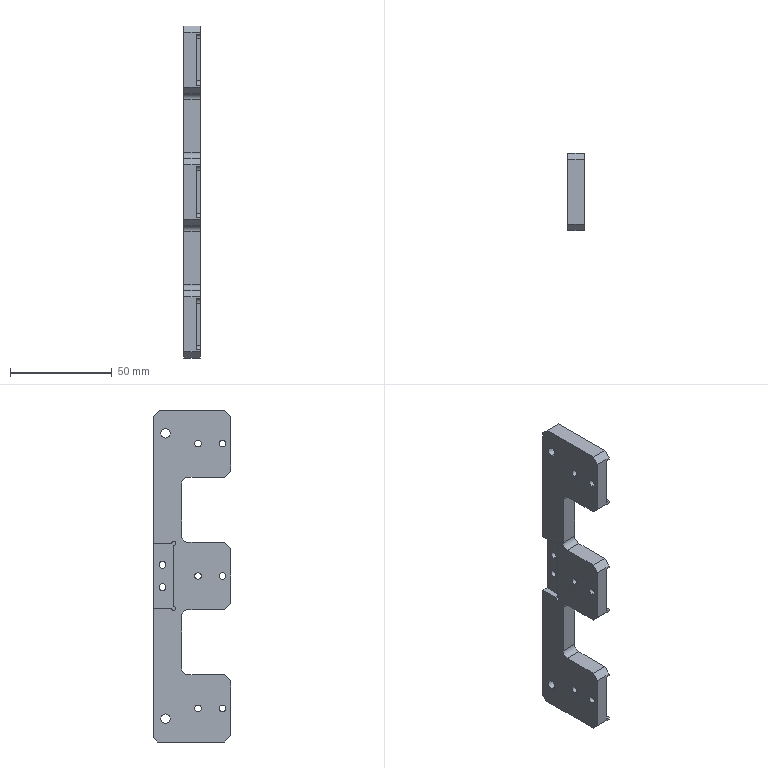Part | STEP file | 0-10-20 Support plate connecting plate | 1 solid | 77 faces | box 8 x 38 x 163 mm | volume 31566 mm3 | plane 40 | cylinder 37 | commonest cylinder face diameters 3.3 x12 4 x6 3.4 x4 4.5 x4 6 x4 8 x4